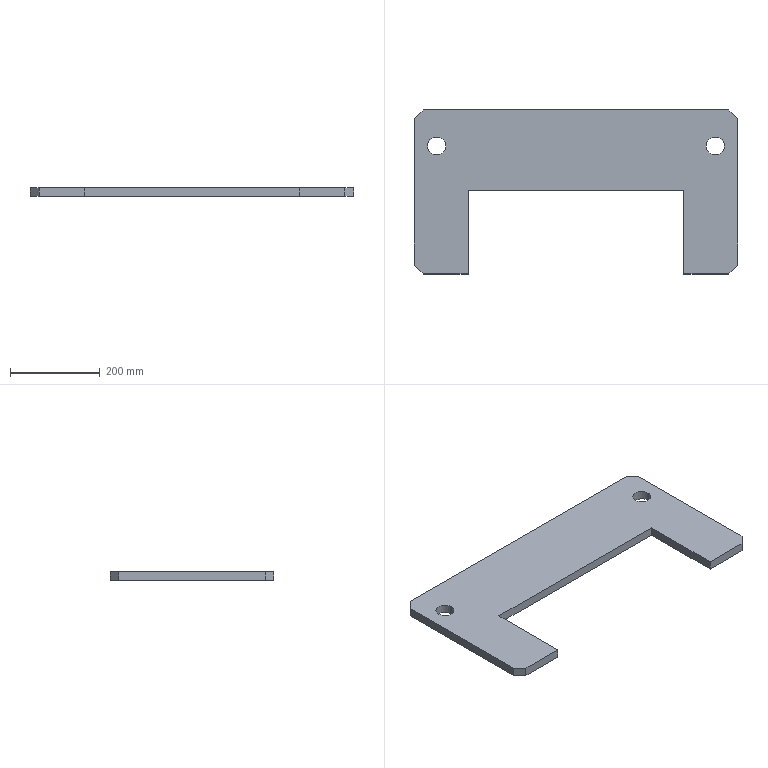Part | SolidWorks | features Chamfer 2, ICE 2, Extrusion 1 | 1 solid | 18 faces | box 720 x 365 x 20 mm | volume 3413735 mm3 | plane 14 | cylinder 4 | commonest cylinder face diameters 40 x4
STEP:
#1=CARTESIAN_POINT('',(-330.,102.5,0.));
#2=VERTEX_POINT('',#1);
#3=CARTESIAN_POINT('',(-290.,102.5,0.));
#4=VERTEX_POINT('',#3);
#5=CARTESIAN_POINT('',(-310.,102.5,0.));
#6=DIRECTION('',(0.,0.,1.));
#7=DIRECTION('',(1.,0.,0.));
#8=AXIS2_PLACEMENT_3D('',#5,#6,#7);
#9=CIRCLE('',#8,20.);
#10=EDGE_CURVE('',#2,#4,#9,.T.);
#11=ORIENTED_EDGE('',*,*,#10,.F.);
#12=CARTESIAN_POINT('',(-330.,102.5,20.));
#13=VERTEX_POINT('',#12);
#14=CARTESIAN_POINT('',(-330.,102.5,0.));
#15=DIRECTION('',(0.,0.,1.));
#16=VECTOR('',#15,1000.);
#17=LINE('',#14,#16);
#18=EDGE_CURVE('',#2,#13,#17,.T.);
#19=ORIENTED_EDGE('',*,*,#18,.T.);
#20=CARTESIAN_POINT('',(-290.,102.5,20.));
#21=VERTEX_POINT('',#20);
#22=CARTESIAN_POINT('',(-310.,102.5,20.));
#23=DIRECTION('',(0.,0.,1.));
#24=DIRECTION('',(1.,0.,0.));
#25=AXIS2_PLACEMENT_3D('',#22,#23,#24);
#26=CIRCLE('',#25,20.);
#27=EDGE_CURVE('',#13,#21,#26,.T.);
#28=ORIENTED_EDGE('',*,*,#27,.T.);
#29=CARTESIAN_POINT('',(-290.,102.5,0.));
#30=DIRECTION('',(0.,0.,1.));
#31=VECTOR('',#30,1000.);
#32=LINE('',#29,#31);
#33=EDGE_CURVE('',#4,#21,#32,.T.);
#34=ORIENTED_EDGE('',*,*,#33,.F.);
#35=EDGE_LOOP('',(#11,#19,#28,#34));
#36=FACE_OUTER_BOUND('',#35,.T.);
#37=CARTESIAN_POINT('',(-310.,102.5,0.));
#38=DIRECTION('',(0.,0.,1.));
#39=DIRECTION('',(1.,0.,0.));
#40=AXIS2_PLACEMENT_3D('',#37,#38,#39);
#41=CYLINDRICAL_SURFACE('',#40,20.);
#42=ADVANCED_FACE('',(#36),#41,.F.);
#43=CARTESIAN_POINT('',(290.,102.5,0.));
#44=VERTEX_POINT('',#43);
#45=CARTESIAN_POINT('',(330.,102.5,0.));
#46=VERTEX_POINT('',#45);
#47=CARTESIAN_POINT('',(310.,102.5,0.));
#48=DIRECTION('',(0.,0.,1.));
#49=DIRECTION('',(-1.,0.,0.));
#50=AXIS2_PLACEMENT_3D('',#47,#48,#49);
#51=CIRCLE('',#50,20.);
#52=EDGE_CURVE('',#44,#46,#51,.T.);
#53=ORIENTED_EDGE('',*,*,#52,.F.);
#54=CARTESIAN_POINT('',(290.,102.5,20.));
#55=VERTEX_POINT('',#54);
#56=CARTESIAN_POINT('',(290.,102.5,0.));
#57=DIRECTION('',(0.,0.,1.));
#58=VECTOR('',#57,1000.);
#59=LINE('',#56,#58);
#60=EDGE_CURVE('',#44,#55,#59,.T.);
#61=ORIENTED_EDGE('',*,*,#60,.T.);
#62=CARTESIAN_POINT('',(330.,102.5,20.));
#63=VERTEX_POINT('',#62);
#64=CARTESIAN_POINT('',(310.,102.5,20.));
#65=DIRECTION('',(0.,0.,1.));
#66=DIRECTION('',(1.,0.,0.));
#67=AXIS2_PLACEMENT_3D('',#64,#65,#66);
#68=CIRCLE('',#67,20.);
#69=EDGE_CURVE('',#55,#63,#68,.T.);
#70=ORIENTED_EDGE('',*,*,#69,.T.);
#71=CARTESIAN_POINT('',(330.,102.5,0.));
#72=DIRECTION('',(0.,0.,1.));
#73=VECTOR('',#72,1000.);
#74=LINE('',#71,#73);
#75=EDGE_CURVE('',#46,#63,#74,.T.);
#76=ORIENTED_EDGE('',*,*,#75,.F.);
#77=EDGE_LOOP('',(#53,#61,#70,#76));
#78=FACE_OUTER_BOUND('',#77,.T.);
#79=CARTESIAN_POINT('',(310.,102.5,0.));
#80=DIRECTION('',(0.,0.,1.));
#81=DIRECTION('',(1.,0.,0.));
#82=AXIS2_PLACEMENT_3D('',#79,#80,#81);
#83=CYLINDRICAL_SURFACE('',#82,20.);
#84=ADVANCED_FACE('',(#78),#83,.F.);
#85=CARTESIAN_POINT('',(240.,-182.5,20.));
#86=VERTEX_POINT('',#85);
#87=CARTESIAN_POINT('',(340.,-182.5,20.));
#88=VERTEX_POINT('',#87);
#89=CARTESIAN_POINT('',(-360.,-182.5,20.));
#90=DIRECTION('',(1.,0.,0.));
#91=VECTOR('',#90,1000.);
#92=LINE('',#89,#91);
#93=EDGE_CURVE('',#86,#88,#92,.T.);
#94=ORIENTED_EDGE('',*,*,#93,.F.);
#95=CARTESIAN_POINT('',(240.,-182.5,0.));
#96=VERTEX_POINT('',#95);
#97=CARTESIAN_POINT('',(240.,-182.5,20.));
#98=DIRECTION('',(0.,0.,-1.));
#99=VECTOR('',#98,1000.);
#100=LINE('',#97,#99);
#101=EDGE_CURVE('',#86,#96,#100,.T.);
#102=ORIENTED_EDGE('',*,*,#101,.T.);
#103=CARTESIAN_POINT('',(340.,-182.5,0.));
#104=VERTEX_POINT('',#103);
#105=CARTESIAN_POINT('',(-360.,-182.5,0.));
#106=DIRECTION('',(1.,0.,0.));
#107=VECTOR('',#106,1000.);
#108=LINE('',#105,#107);
#109=EDGE_CURVE('',#96,#104,#108,.T.);
#110=ORIENTED_EDGE('',*,*,#109,.T.);
#111=CARTESIAN_POINT('',(340.,-182.5,20.));
#112=DIRECTION('',(0.,0.,1.));
#113=VECTOR('',#112,1000.);
#114=LINE('',#111,#113);
#115=EDGE_CURVE('',#104,#88,#114,.T.);
#116=ORIENTED_EDGE('',*,*,#115,.T.);
#117=EDGE_LOOP('',(#94,#102,#110,#116));
#118=FACE_OUTER_BOUND('',#117,.T.);
#119=CARTESIAN_POINT('',(-360.,-182.5,20.));
#120=DIRECTION('',(0.,1.,0.));
#121=DIRECTION('',(0.,0.,1.));
#122=AXIS2_PLACEMENT_3D('',#119,#120,#121);
#123=PLANE('',#122);
#124=ADVANCED_FACE('',(#118),#123,.F.);
#125=CARTESIAN_POINT('',(360.,-162.5,20.));
#126=VERTEX_POINT('',#125);
#127=CARTESIAN_POINT('',(360.,162.5,20.));
#128=VERTEX_POINT('',#127);
#129=CARTESIAN_POINT('',(360.,182.5,20.));
#130=DIRECTION('',(0.,1.,0.));
#131=VECTOR('',#130,1000.);
#132=LINE('',#129,#131);
#133=EDGE_CURVE('',#126,#128,#132,.T.);
#134=ORIENTED_EDGE('',*,*,#133,.F.);
#135=CARTESIAN_POINT('',(360.,-162.5,0.));
#136=VERTEX_POINT('',#135);
#137=CARTESIAN_POINT('',(360.,-162.5,20.));
#138=DIRECTION('',(0.,0.,-1.));
#139=VECTOR('',#138,1000.);
#140=LINE('',#137,#139);
#141=EDGE_CURVE('',#126,#136,#140,.T.);
#142=ORIENTED_EDGE('',*,*,#141,.T.);
#143=CARTESIAN_POINT('',(360.,162.5,0.));
#144=VERTEX_POINT('',#143);
#145=CARTESIAN_POINT('',(360.,182.5,0.));
#146=DIRECTION('',(0.,1.,0.));
#147=VECTOR('',#146,1000.);
#148=LINE('',#145,#147);
#149=EDGE_CURVE('',#136,#144,#148,.T.);
#150=ORIENTED_EDGE('',*,*,#149,.T.);
#151=CARTESIAN_POINT('',(360.,162.5,20.));
#152=DIRECTION('',(0.,0.,1.));
#153=VECTOR('',#152,1000.);
#154=LINE('',#151,#153);
#155=EDGE_CURVE('',#144,#128,#154,.T.);
#156=ORIENTED_EDGE('',*,*,#155,.T.);
#157=EDGE_LOOP('',(#134,#142,#150,#156));
#158=FACE_OUTER_BOUND('',#157,.T.);
#159=CARTESIAN_POINT('',(360.,182.5,20.));
#160=DIRECTION('',(-1.,0.,0.));
#161=DIRECTION('',(0.,-1.,0.));
#162=AXIS2_PLACEMENT_3D('',#159,#160,#161);
#163=PLANE('',#162);
#164=ADVANCED_FACE('',(#158),#163,.F.);
#165=CARTESIAN_POINT('',(340.,182.5,0.));
#166=VERTEX_POINT('',#165);
#167=CARTESIAN_POINT('',(-340.,182.5,0.));
#168=VERTEX_POINT('',#167);
#169=CARTESIAN_POINT('',(-360.,182.5,0.));
#170=DIRECTION('',(-1.,0.,0.));
#171=VECTOR('',#170,1000.);
#172=LINE('',#169,#171);
#173=EDGE_CURVE('',#166,#168,#172,.T.);
#174=ORIENTED_EDGE('',*,*,#173,.T.);
#175=CARTESIAN_POINT('',(-340.,182.5,20.));
#176=VERTEX_POINT('',#175);
#177=CARTESIAN_POINT('',(-340.,182.5,20.));
#178=DIRECTION('',(0.,0.,1.));
#179=VECTOR('',#178,1000.);
#180=LINE('',#177,#179);
#181=EDGE_CURVE('',#168,#176,#180,.T.);
#182=ORIENTED_EDGE('',*,*,#181,.T.);
#183=CARTESIAN_POINT('',(340.,182.5,20.));
#184=VERTEX_POINT('',#183);
#185=CARTESIAN_POINT('',(-360.,182.5,20.));
#186=DIRECTION('',(-1.,0.,0.));
#187=VECTOR('',#186,1000.);
#188=LINE('',#185,#187);
#189=EDGE_CURVE('',#184,#176,#188,.T.);
#190=ORIENTED_EDGE('',*,*,#189,.F.);
#191=CARTESIAN_POINT('',(340.,182.5,20.));
#192=DIRECTION('',(0.,0.,-1.));
#193=VECTOR('',#192,1000.);
#194=LINE('',#191,#193);
#195=EDGE_CURVE('',#184,#166,#194,.T.);
#196=ORIENTED_EDGE('',*,*,#195,.T.);
#197=EDGE_LOOP('',(#174,#182,#190,#196));
#198=FACE_OUTER_BOUND('',#197,.T.);
#199=CARTESIAN_POINT('',(-360.,182.5,20.));
#200=DIRECTION('',(0.,-1.,0.));
#201=DIRECTION('',(1.,0.,0.));
#202=AXIS2_PLACEMENT_3D('',#199,#200,#201);
#203=PLANE('',#202);
#204=ADVANCED_FACE('',(#198),#203,.F.);
#205=CARTESIAN_POINT('',(-360.,162.5,0.));
#206=VERTEX_POINT('',#205);
#207=CARTESIAN_POINT('',(-360.,-162.5,0.));
#208=VERTEX_POINT('',#207);
#209=CARTESIAN_POINT('',(-360.,182.5,0.));
#210=DIRECTION('',(0.,-1.,0.));
#211=VECTOR('',#210,1000.);
#212=LINE('',#209,#211);
#213=EDGE_CURVE('',#206,#208,#212,.T.);
#214=ORIENTED_EDGE('',*,*,#213,.T.);
#215=CARTESIAN_POINT('',(-360.,-162.5,20.));
#216=VERTEX_POINT('',#215);
#217=CARTESIAN_POINT('',(-360.,-162.5,20.));
#218=DIRECTION('',(0.,0.,1.));
#219=VECTOR('',#218,1000.);
#220=LINE('',#217,#219);
#221=EDGE_CURVE('',#208,#216,#220,.T.);
#222=ORIENTED_EDGE('',*,*,#221,.T.);
#223=CARTESIAN_POINT('',(-360.,162.5,20.));
#224=VERTEX_POINT('',#223);
#225=CARTESIAN_POINT('',(-360.,182.5,20.));
#226=DIRECTION('',(0.,-1.,0.));
#227=VECTOR('',#226,1000.);
#228=LINE('',#225,#227);
#229=EDGE_CURVE('',#224,#216,#228,.T.);
#230=ORIENTED_EDGE('',*,*,#229,.F.);
#231=CARTESIAN_POINT('',(-360.,162.5,20.));
#232=DIRECTION('',(0.,0.,-1.));
#233=VECTOR('',#232,1000.);
#234=LINE('',#231,#233);
#235=EDGE_CURVE('',#224,#206,#234,.T.);
#236=ORIENTED_EDGE('',*,*,#235,.T.);
#237=EDGE_LOOP('',(#214,#222,#230,#236));
#238=FACE_OUTER_BOUND('',#237,.T.);
#239=CARTESIAN_POINT('',(-360.,182.5,20.));
#240=DIRECTION('',(1.,0.,0.));
#241=DIRECTION('',(0.,1.,0.));
#242=AXIS2_PLACEMENT_3D('',#239,#240,#241);
#243=PLANE('',#242);
#244=ADVANCED_FACE('',(#238),#243,.F.);
#245=CARTESIAN_POINT('',(-340.,-182.5,0.));
#246=VERTEX_POINT('',#245);
#247=CARTESIAN_POINT('',(-240.,-182.5,0.));
#248=VERTEX_POINT('',#247);
#249=CARTESIAN_POINT('',(-360.,-182.5,0.));
#250=DIRECTION('',(1.,0.,0.));
#251=VECTOR('',#250,1000.);
#252=LINE('',#249,#251);
#253=EDGE_CURVE('',#246,#248,#252,.T.);
#254=ORIENTED_EDGE('',*,*,#253,.T.);
#255=CARTESIAN_POINT('',(-240.,-182.5,20.));
#256=VERTEX_POINT('',#255);
#257=CARTESIAN_POINT('',(-240.,-182.5,20.));
#258=DIRECTION('',(0.,0.,1.));
#259=VECTOR('',#258,1000.);
#260=LINE('',#257,#259);
#261=EDGE_CURVE('',#248,#256,#260,.T.);
#262=ORIENTED_EDGE('',*,*,#261,.T.);
#263=CARTESIAN_POINT('',(-340.,-182.5,20.));
#264=VERTEX_POINT('',#263);
#265=CARTESIAN_POINT('',(-360.,-182.5,20.));
#266=DIRECTION('',(1.,0.,0.));
#267=VECTOR('',#266,1000.);
#268=LINE('',#265,#267);
#269=EDGE_CURVE('',#264,#256,#268,.T.);
#270=ORIENTED_EDGE('',*,*,#269,.F.);
#271=CARTESIAN_POINT('',(-340.,-182.5,20.));
#272=DIRECTION('',(0.,0.,-1.));
#273=VECTOR('',#272,1000.);
#274=LINE('',#271,#273);
#275=EDGE_CURVE('',#264,#246,#274,.T.);
#276=ORIENTED_EDGE('',*,*,#275,.T.);
#277=EDGE_LOOP('',(#254,#262,#270,#276));
#278=FACE_OUTER_BOUND('',#277,.T.);
#279=CARTESIAN_POINT('',(-360.,-182.5,20.));
#280=DIRECTION('',(0.,1.,0.));
#281=DIRECTION('',(0.,0.,1.));
#282=AXIS2_PLACEMENT_3D('',#279,#280,#281);
#283=PLANE('',#282);
#284=ADVANCED_FACE('',(#278),#283,.F.);
#285=CARTESIAN_POINT('',(240.,2.5,20.));
#286=VERTEX_POINT('',#285);
#287=CARTESIAN_POINT('',(240.,0.,20.));
#288=DIRECTION('',(0.,1.,0.));
#289=VECTOR('',#288,1000.);
#290=LINE('',#287,#289);
#291=EDGE_CURVE('',#86,#286,#290,.T.);
#292=ORIENTED_EDGE('',*,*,#291,.F.);
#293=ORIENTED_EDGE('',*,*,#93,.T.);
#294=CARTESIAN_POINT('',(261.25,-261.25,20.));
#295=DIRECTION('',(0.7071,0.7071,0.));
#296=VECTOR('',#295,1000.);
#297=LINE('',#294,#296);
#298=EDGE_CURVE('',#88,#126,#297,.T.);
#299=ORIENTED_EDGE('',*,*,#298,.T.);
#300=ORIENTED_EDGE('',*,*,#133,.T.);
#301=CARTESIAN_POINT('',(261.25,261.25,20.));
#302=DIRECTION('',(-0.7071,0.7071,0.));
#303=VECTOR('',#302,1000.);
#304=LINE('',#301,#303);
#305=EDGE_CURVE('',#128,#184,#304,.T.);
#306=ORIENTED_EDGE('',*,*,#305,.T.);
#307=ORIENTED_EDGE('',*,*,#189,.T.);
#308=CARTESIAN_POINT('',(-261.25,261.25,20.));
#309=DIRECTION('',(-0.7071,-0.7071,0.));
#310=VECTOR('',#309,1000.);
#311=LINE('',#308,#310);
#312=EDGE_CURVE('',#176,#224,#311,.T.);
#313=ORIENTED_EDGE('',*,*,#312,.T.);
#314=ORIENTED_EDGE('',*,*,#229,.T.);
#315=CARTESIAN_POINT('',(-261.25,-261.25,20.));
#316=DIRECTION('',(0.7071,-0.7071,0.));
#317=VECTOR('',#316,1000.);
#318=LINE('',#315,#317);
#319=EDGE_CURVE('',#216,#264,#318,.T.);
#320=ORIENTED_EDGE('',*,*,#319,.T.);
#321=ORIENTED_EDGE('',*,*,#269,.T.);
#322=CARTESIAN_POINT('',(-240.,2.5,20.));
#323=VERTEX_POINT('',#322);
#324=CARTESIAN_POINT('',(-240.,0.,20.));
#325=DIRECTION('',(0.,-1.,0.));
#326=VECTOR('',#325,1000.);
#327=LINE('',#324,#326);
#328=EDGE_CURVE('',#323,#256,#327,.T.);
#329=ORIENTED_EDGE('',*,*,#328,.F.);
#330=CARTESIAN_POINT('',(0.,2.5,20.));
#331=DIRECTION('',(-1.,0.,0.));
#332=VECTOR('',#331,1000.);
#333=LINE('',#330,#332);
#334=EDGE_CURVE('',#286,#323,#333,.T.);
#335=ORIENTED_EDGE('',*,*,#334,.F.);
#336=EDGE_LOOP('',(#292,#293,#299,#300,#306,#307,#313,#314,#320,#321,#329,#335));
#337=FACE_OUTER_BOUND('',#336,.T.);
#338=CARTESIAN_POINT('',(-310.,102.5,20.));
#339=DIRECTION('',(0.,0.,1.));
#340=DIRECTION('',(1.,0.,0.));
#341=AXIS2_PLACEMENT_3D('',#338,#339,#340);
#342=CIRCLE('',#341,20.);
#343=EDGE_CURVE('',#21,#13,#342,.T.);
#344=ORIENTED_EDGE('',*,*,#343,.F.);
#345=ORIENTED_EDGE('',*,*,#27,.F.);
#346=EDGE_LOOP('',(#344,#345));
#347=FACE_BOUND('',#346,.T.);
#348=CARTESIAN_POINT('',(310.,102.5,20.));
#349=DIRECTION('',(0.,0.,1.));
#350=DIRECTION('',(1.,0.,0.));
#351=AXIS2_PLACEMENT_3D('',#348,#349,#350);
#352=CIRCLE('',#351,20.);
#353=EDGE_CURVE('',#63,#55,#352,.T.);
#354=ORIENTED_EDGE('',*,*,#353,.F.);
#355=ORIENTED_EDGE('',*,*,#69,.F.);
#356=EDGE_LOOP('',(#354,#355));
#357=FACE_BOUND('',#356,.T.);
#358=CARTESIAN_POINT('',(0.,0.,20.));
#359=DIRECTION('',(0.,0.,1.));
#360=DIRECTION('',(1.,0.,0.));
#361=AXIS2_PLACEMENT_3D('',#358,#359,#360);
#362=PLANE('',#361);
#363=ADVANCED_FACE('',(#337,#347,#357),#362,.T.);
#364=ORIENTED_EDGE('',*,*,#109,.F.);
#365=CARTESIAN_POINT('',(240.,2.5,0.));
#366=VERTEX_POINT('',#365);
#367=CARTESIAN_POINT('',(240.,0.,0.));
#368=DIRECTION('',(0.,1.,0.));
#369=VECTOR('',#368,1000.);
#370=LINE('',#367,#369);
#371=EDGE_CURVE('',#96,#366,#370,.T.);
#372=ORIENTED_EDGE('',*,*,#371,.T.);
#373=CARTESIAN_POINT('',(-240.,2.5,0.));
#374=VERTEX_POINT('',#373);
#375=CARTESIAN_POINT('',(-240.,2.5,0.));
#376=DIRECTION('',(-1.,0.,0.));
#377=VECTOR('',#376,1000.);
#378=LINE('',#375,#377);
#379=EDGE_CURVE('',#366,#374,#378,.T.);
#380=ORIENTED_EDGE('',*,*,#379,.T.);
#381=CARTESIAN_POINT('',(-240.,2.5,0.));
#382=DIRECTION('',(0.,-1.,0.));
#383=VECTOR('',#382,1000.);
#384=LINE('',#381,#383);
#385=EDGE_CURVE('',#374,#248,#384,.T.);
#386=ORIENTED_EDGE('',*,*,#385,.T.);
#387=ORIENTED_EDGE('',*,*,#253,.F.);
#388=CARTESIAN_POINT('',(-340.,-182.5,0.));
#389=DIRECTION('',(-0.7071,0.7071,0.));
#390=VECTOR('',#389,1000.);
#391=LINE('',#388,#390);
#392=EDGE_CURVE('',#246,#208,#391,.T.);
#393=ORIENTED_EDGE('',*,*,#392,.T.);
#394=ORIENTED_EDGE('',*,*,#213,.F.);
#395=CARTESIAN_POINT('',(-360.,162.5,0.));
#396=DIRECTION('',(0.7071,0.7071,0.));
#397=VECTOR('',#396,1000.);
#398=LINE('',#395,#397);
#399=EDGE_CURVE('',#206,#168,#398,.T.);
#400=ORIENTED_EDGE('',*,*,#399,.T.);
#401=ORIENTED_EDGE('',*,*,#173,.F.);
#402=CARTESIAN_POINT('',(340.,182.5,0.));
#403=DIRECTION('',(0.7071,-0.7071,0.));
#404=VECTOR('',#403,1000.);
#405=LINE('',#402,#404);
#406=EDGE_CURVE('',#166,#144,#405,.T.);
#407=ORIENTED_EDGE('',*,*,#406,.T.);
#408=ORIENTED_EDGE('',*,*,#149,.F.);
#409=CARTESIAN_POINT('',(360.,-162.5,0.));
#410=DIRECTION('',(-0.7071,-0.7071,0.));
#411=VECTOR('',#410,1000.);
#412=LINE('',#409,#411);
#413=EDGE_CURVE('',#136,#104,#412,.T.);
#414=ORIENTED_EDGE('',*,*,#413,.T.);
#415=EDGE_LOOP('',(#364,#372,#380,#386,#387,#393,#394,#400,#401,#407,#408,#414));
#416=FACE_OUTER_BOUND('',#415,.T.);
#417=CARTESIAN_POINT('',(-310.,102.5,0.));
#418=DIRECTION('',(0.,0.,1.));
#419=DIRECTION('',(1.,0.,0.));
#420=AXIS2_PLACEMENT_3D('',#417,#418,#419);
#421=CIRCLE('',#420,20.);
#422=EDGE_CURVE('',#4,#2,#421,.T.);
#423=ORIENTED_EDGE('',*,*,#422,.T.);
#424=ORIENTED_EDGE('',*,*,#10,.T.);
#425=EDGE_LOOP('',(#423,#424));
#426=FACE_BOUND('',#425,.T.);
#427=CARTESIAN_POINT('',(310.,102.5,0.));
#428=DIRECTION('',(0.,0.,1.));
#429=DIRECTION('',(-1.,0.,0.));
#430=AXIS2_PLACEMENT_3D('',#427,#428,#429);
#431=CIRCLE('',#430,20.);
#432=EDGE_CURVE('',#46,#44,#431,.T.);
#433=ORIENTED_EDGE('',*,*,#432,.T.);
#434=ORIENTED_EDGE('',*,*,#52,.T.);
#435=EDGE_LOOP('',(#433,#434));
#436=FACE_BOUND('',#435,.T.);
#437=CARTESIAN_POINT('',(0.,0.,0.));
#438=DIRECTION('',(0.,0.,1.));
#439=DIRECTION('',(1.,0.,0.));
#440=AXIS2_PLACEMENT_3D('',#437,#438,#439);
#441=PLANE('',#440);
#442=ADVANCED_FACE('',(#416,#426,#436),#441,.F.);
#443=ORIENTED_EDGE('',*,*,#60,.F.);
#444=ORIENTED_EDGE('',*,*,#432,.F.);
#445=ORIENTED_EDGE('',*,*,#75,.T.);
#446=ORIENTED_EDGE('',*,*,#353,.T.);
#447=EDGE_LOOP('',(#443,#444,#445,#446));
#448=FACE_OUTER_BOUND('',#447,.T.);
#449=CARTESIAN_POINT('',(310.,102.5,0.));
#450=DIRECTION('',(0.,0.,1.));
#451=DIRECTION('',(1.,0.,0.));
#452=AXIS2_PLACEMENT_3D('',#449,#450,#451);
#453=CYLINDRICAL_SURFACE('',#452,20.);
#454=ADVANCED_FACE('',(#448),#453,.F.);
#455=ORIENTED_EDGE('',*,*,#18,.F.);
#456=ORIENTED_EDGE('',*,*,#422,.F.);
#457=ORIENTED_EDGE('',*,*,#33,.T.);
#458=ORIENTED_EDGE('',*,*,#343,.T.);
#459=EDGE_LOOP('',(#455,#456,#457,#458));
#460=FACE_OUTER_BOUND('',#459,.T.);
#461=CARTESIAN_POINT('',(-310.,102.5,0.));
#462=DIRECTION('',(0.,0.,1.));
#463=DIRECTION('',(1.,0.,0.));
#464=AXIS2_PLACEMENT_3D('',#461,#462,#463);
#465=CYLINDRICAL_SURFACE('',#464,20.);
#466=ADVANCED_FACE('',(#460),#465,.F.);
#467=ORIENTED_EDGE('',*,*,#312,.F.);
#468=ORIENTED_EDGE('',*,*,#181,.F.);
#469=ORIENTED_EDGE('',*,*,#399,.F.);
#470=ORIENTED_EDGE('',*,*,#235,.F.);
#471=EDGE_LOOP('',(#467,#468,#469,#470));
#472=FACE_OUTER_BOUND('',#471,.T.);
#473=CARTESIAN_POINT('',(-360.,162.5,20.));
#474=DIRECTION('',(0.7071,-0.7071,0.));
#475=DIRECTION('',(0.,0.,-1.));
#476=AXIS2_PLACEMENT_3D('',#473,#474,#475);
#477=PLANE('',#476);
#478=ADVANCED_FACE('',(#472),#477,.F.);
#479=ORIENTED_EDGE('',*,*,#305,.F.);
#480=ORIENTED_EDGE('',*,*,#155,.F.);
#481=ORIENTED_EDGE('',*,*,#406,.F.);
#482=ORIENTED_EDGE('',*,*,#195,.F.);
#483=EDGE_LOOP('',(#479,#480,#481,#482));
#484=FACE_OUTER_BOUND('',#483,.T.);
#485=CARTESIAN_POINT('',(340.,182.5,20.));
#486=DIRECTION('',(-0.7071,-0.7071,0.));
#487=DIRECTION('',(0.,0.,-1.));
#488=AXIS2_PLACEMENT_3D('',#485,#486,#487);
#489=PLANE('',#488);
#490=ADVANCED_FACE('',(#484),#489,.F.);
#491=ORIENTED_EDGE('',*,*,#298,.F.);
#492=ORIENTED_EDGE('',*,*,#115,.F.);
#493=ORIENTED_EDGE('',*,*,#413,.F.);
#494=ORIENTED_EDGE('',*,*,#141,.F.);
#495=EDGE_LOOP('',(#491,#492,#493,#494));
#496=FACE_OUTER_BOUND('',#495,.T.);
#497=CARTESIAN_POINT('',(360.,-162.5,20.));
#498=DIRECTION('',(-0.7071,0.7071,0.));
#499=DIRECTION('',(0.,0.,-1.));
#500=AXIS2_PLACEMENT_3D('',#497,#498,#499);
#501=PLANE('',#500);
#502=ADVANCED_FACE('',(#496),#501,.F.);
#503=ORIENTED_EDGE('',*,*,#319,.F.);
#504=ORIENTED_EDGE('',*,*,#221,.F.);
#505=ORIENTED_EDGE('',*,*,#392,.F.);
#506=ORIENTED_EDGE('',*,*,#275,.F.);
#507=EDGE_LOOP('',(#503,#504,#505,#506));
#508=FACE_OUTER_BOUND('',#507,.T.);
#509=CARTESIAN_POINT('',(-340.,-182.5,20.));
#510=DIRECTION('',(0.7071,0.7071,0.));
#511=DIRECTION('',(0.,0.,-1.));
#512=AXIS2_PLACEMENT_3D('',#509,#510,#511);
#513=PLANE('',#512);
#514=ADVANCED_FACE('',(#508),#513,.F.);
#515=ORIENTED_EDGE('',*,*,#291,.T.);
#516=CARTESIAN_POINT('',(240.,2.5,0.));
#517=DIRECTION('',(0.,0.,1.));
#518=VECTOR('',#517,1000.);
#519=LINE('',#516,#518);
#520=EDGE_CURVE('',#366,#286,#519,.T.);
#521=ORIENTED_EDGE('',*,*,#520,.F.);
#522=ORIENTED_EDGE('',*,*,#371,.F.);
#523=ORIENTED_EDGE('',*,*,#101,.F.);
#524=EDGE_LOOP('',(#515,#521,#522,#523));
#525=FACE_OUTER_BOUND('',#524,.T.);
#526=CARTESIAN_POINT('',(240.,2.5,0.));
#527=DIRECTION('',(1.,0.,0.));
#528=DIRECTION('',(0.,1.,0.));
#529=AXIS2_PLACEMENT_3D('',#526,#527,#528);
#530=PLANE('',#529);
#531=ADVANCED_FACE('',(#525),#530,.F.);
#532=ORIENTED_EDGE('',*,*,#385,.F.);
#533=CARTESIAN_POINT('',(-240.,2.5,0.));
#534=DIRECTION('',(0.,0.,1.));
#535=VECTOR('',#534,1000.);
#536=LINE('',#533,#535);
#537=EDGE_CURVE('',#374,#323,#536,.T.);
#538=ORIENTED_EDGE('',*,*,#537,.T.);
#539=ORIENTED_EDGE('',*,*,#328,.T.);
#540=ORIENTED_EDGE('',*,*,#261,.F.);
#541=EDGE_LOOP('',(#532,#538,#539,#540));
#542=FACE_OUTER_BOUND('',#541,.T.);
#543=CARTESIAN_POINT('',(-240.,2.5,0.));
#544=DIRECTION('',(-1.,0.,0.));
#545=DIRECTION('',(0.,-1.,0.));
#546=AXIS2_PLACEMENT_3D('',#543,#544,#545);
#547=PLANE('',#546);
#548=ADVANCED_FACE('',(#542),#547,.F.);
#549=ORIENTED_EDGE('',*,*,#334,.T.);
#550=ORIENTED_EDGE('',*,*,#537,.F.);
#551=ORIENTED_EDGE('',*,*,#379,.F.);
#552=ORIENTED_EDGE('',*,*,#520,.T.);
#553=EDGE_LOOP('',(#549,#550,#551,#552));
#554=FACE_OUTER_BOUND('',#553,.T.);
#555=CARTESIAN_POINT('',(-240.,2.5,0.));
#556=DIRECTION('',(0.,1.,0.));
#557=DIRECTION('',(0.,0.,1.));
#558=AXIS2_PLACEMENT_3D('',#555,#556,#557);
#559=PLANE('',#558);
#560=ADVANCED_FACE('',(#554),#559,.F.);
#561=CLOSED_SHELL('',(#42,#84,#124,#164,#204,#244,#284,#363,#442,#454,#466,#478,#490,#502,#514,#531,#548,#560));
#562=MANIFOLD_SOLID_BREP('',#561);
#563=CARTESIAN_POINT('',(0.,0.,0.));
#564=DIRECTION('',(0.,0.,1.));
#565=DIRECTION('',(1.,0.,0.));
#566=AXIS2_PLACEMENT_3D('',#563,#564,#565);
#567=(LENGTH_UNIT()NAMED_UNIT(*)SI_UNIT(.MILLI.,.METRE.));
#568=UNCERTAINTY_MEASURE_WITH_UNIT(LENGTH_MEASURE(0.00001),#567,'','');
#569=(NAMED_UNIT(*)PLANE_ANGLE_UNIT()SI_UNIT($,.RADIAN.));
#570=(NAMED_UNIT(*)SI_UNIT($,.STERADIAN.)SOLID_ANGLE_UNIT());
#571=(GEOMETRIC_REPRESENTATION_CONTEXT(3)GLOBAL_UNCERTAINTY_ASSIGNED_CONTEXT((#568))GLOBAL_UNIT_ASSIGNED_CONTEXT((#567,#569,#570))REPRESENTATION_CONTEXT('',''));
#572=ADVANCED_BREP_SHAPE_REPRESENTATION('',(#562,#566),#571);